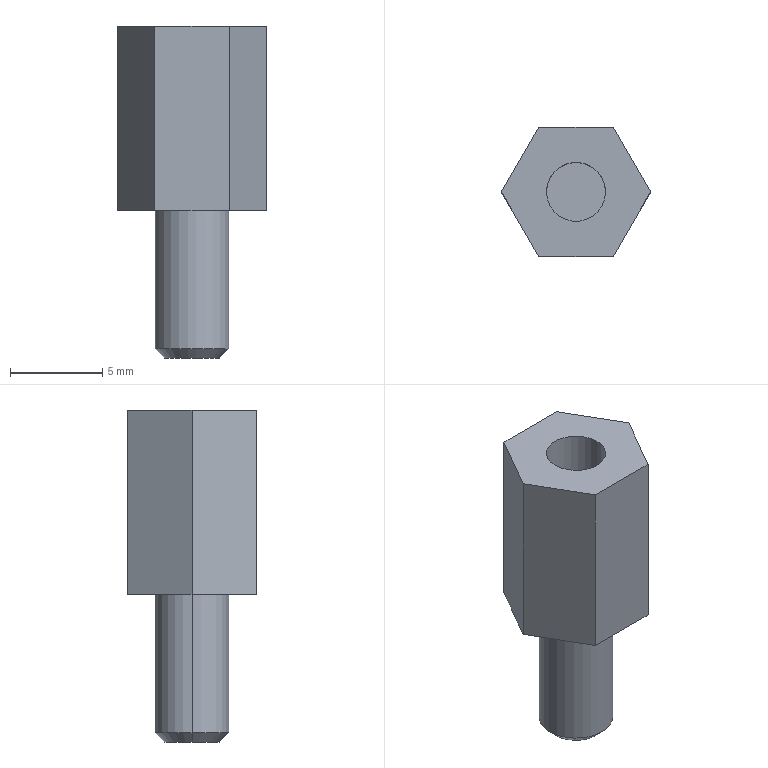Part | STEP file | 58411934 | 1 solid | 16 faces | box 8.091 x 7 x 18 mm | volume 467.745 mm3 | plane 10 | cylinder 4 | cone 2 | commonest cylinder face diameters 3.2 x2 4 x2
STEP:
#1=CARTESIAN_POINT('',(0.,0.,0.));
#2=DIRECTION('',(0.,0.,1.));
#3=DIRECTION('',(1.,0.,0.));
#4=AXIS2_PLACEMENT_3D('',#1,#2,#3);
#5=CARTESIAN_POINT('',(-2.025,3.5,0.));
#6=VERTEX_POINT('',#5);
#7=CARTESIAN_POINT('',(-4.046,0.,0.));
#8=VERTEX_POINT('',#7);
#9=CARTESIAN_POINT('',(-2.025,3.5,0.));
#10=DIRECTION('',(-0.5,-0.866,0.));
#11=VECTOR('',#10,1.);
#12=LINE('',#9,#11);
#13=CARTESIAN_POINT('',(0.,0.,0.));
#14=DIRECTION('',(0.,0.,1.));
#15=DIRECTION('',(1.,0.,0.));
#16=AXIS2_PLACEMENT_3D('',#13,#14,#15);
#17=PLANE('',#16);
#18=CARTESIAN_POINT('',(-2.025,3.5));
#19=DIRECTION('',(-0.5,-0.866));
#20=VECTOR('',#19,1.);
#21=LINE('',#18,#20);
#22=(GEOMETRIC_REPRESENTATION_CONTEXT(2)PARAMETRIC_REPRESENTATION_CONTEXT()REPRESENTATION_CONTEXT('',''));
#23=DEFINITIONAL_REPRESENTATION('',(#21),#22);
#24=PCURVE('',#17,#23);
#25=CARTESIAN_POINT('',(-2.025,3.5,0.));
#26=DIRECTION('',(-0.866,0.5,0.));
#27=DIRECTION('',(-0.5,-0.866,0.));
#28=AXIS2_PLACEMENT_3D('',#25,#26,#27);
#29=PLANE('',#28);
#30=CARTESIAN_POINT('',(0.,0.));
#31=DIRECTION('',(1.,0.));
#32=VECTOR('',#31,1.);
#33=LINE('',#30,#32);
#34=(GEOMETRIC_REPRESENTATION_CONTEXT(2)PARAMETRIC_REPRESENTATION_CONTEXT()REPRESENTATION_CONTEXT('',''));
#35=DEFINITIONAL_REPRESENTATION('',(#33),#34);
#36=PCURVE('',#29,#35);
#37=SURFACE_CURVE('',#12,(#24,#36),.PCURVE_S1.);
#38=EDGE_CURVE('',#6,#8,#37,.T.);
#39=ORIENTED_EDGE('',*,*,#38,.T.);
#40=CARTESIAN_POINT('',(-2.025,-3.5,0.));
#41=VERTEX_POINT('',#40);
#42=CARTESIAN_POINT('',(-2.025,-3.5,0.));
#43=DIRECTION('',(-0.5,0.866,0.));
#44=VECTOR('',#43,1.);
#45=LINE('',#42,#44);
#46=CARTESIAN_POINT('',(-2.025,-3.5));
#47=DIRECTION('',(-0.5,0.866));
#48=VECTOR('',#47,1.);
#49=LINE('',#46,#48);
#50=(GEOMETRIC_REPRESENTATION_CONTEXT(2)PARAMETRIC_REPRESENTATION_CONTEXT()REPRESENTATION_CONTEXT('',''));
#51=DEFINITIONAL_REPRESENTATION('',(#49),#50);
#52=PCURVE('',#17,#51);
#53=CARTESIAN_POINT('',(-2.025,-3.5,0.));
#54=DIRECTION('',(0.866,0.5,0.));
#55=DIRECTION('',(-0.5,0.866,0.));
#56=AXIS2_PLACEMENT_3D('',#53,#54,#55);
#57=PLANE('',#56);
#58=CARTESIAN_POINT('',(0.,0.));
#59=DIRECTION('',(1.,0.));
#60=VECTOR('',#59,1.);
#61=LINE('',#58,#60);
#62=(GEOMETRIC_REPRESENTATION_CONTEXT(2)PARAMETRIC_REPRESENTATION_CONTEXT()REPRESENTATION_CONTEXT('',''));
#63=DEFINITIONAL_REPRESENTATION('',(#61),#62);
#64=PCURVE('',#57,#63);
#65=SURFACE_CURVE('',#45,(#52,#64),.PCURVE_S1.);
#66=EDGE_CURVE('',#41,#8,#65,.T.);
#67=ORIENTED_EDGE('',*,*,#66,.F.);
#68=CARTESIAN_POINT('',(2.025,-3.5,0.));
#69=VERTEX_POINT('',#68);
#70=CARTESIAN_POINT('',(2.025,-3.5,0.));
#71=DIRECTION('',(-1.,0.,0.));
#72=VECTOR('',#71,1.);
#73=LINE('',#70,#72);
#74=CARTESIAN_POINT('',(2.025,-3.5));
#75=DIRECTION('',(-1.,0.));
#76=VECTOR('',#75,1.);
#77=LINE('',#74,#76);
#78=(GEOMETRIC_REPRESENTATION_CONTEXT(2)PARAMETRIC_REPRESENTATION_CONTEXT()REPRESENTATION_CONTEXT('',''));
#79=DEFINITIONAL_REPRESENTATION('',(#77),#78);
#80=PCURVE('',#17,#79);
#81=CARTESIAN_POINT('',(2.025,-3.5,0.));
#82=DIRECTION('',(0.,1.,0.));
#83=DIRECTION('',(-1.,0.,0.));
#84=AXIS2_PLACEMENT_3D('',#81,#82,#83);
#85=PLANE('',#84);
#86=CARTESIAN_POINT('',(0.,0.));
#87=DIRECTION('',(1.,0.));
#88=VECTOR('',#87,1.);
#89=LINE('',#86,#88);
#90=(GEOMETRIC_REPRESENTATION_CONTEXT(2)PARAMETRIC_REPRESENTATION_CONTEXT()REPRESENTATION_CONTEXT('',''));
#91=DEFINITIONAL_REPRESENTATION('',(#89),#90);
#92=PCURVE('',#85,#91);
#93=SURFACE_CURVE('',#73,(#80,#92),.PCURVE_S1.);
#94=EDGE_CURVE('',#69,#41,#93,.T.);
#95=ORIENTED_EDGE('',*,*,#94,.F.);
#96=CARTESIAN_POINT('',(4.046,0.,0.));
#97=VERTEX_POINT('',#96);
#98=CARTESIAN_POINT('',(4.046,0.,0.));
#99=DIRECTION('',(-0.5,-0.866,0.));
#100=VECTOR('',#99,1.);
#101=LINE('',#98,#100);
#102=CARTESIAN_POINT('',(4.046,0.));
#103=DIRECTION('',(-0.5,-0.866));
#104=VECTOR('',#103,1.);
#105=LINE('',#102,#104);
#106=(GEOMETRIC_REPRESENTATION_CONTEXT(2)PARAMETRIC_REPRESENTATION_CONTEXT()REPRESENTATION_CONTEXT('',''));
#107=DEFINITIONAL_REPRESENTATION('',(#105),#106);
#108=PCURVE('',#17,#107);
#109=CARTESIAN_POINT('',(4.046,0.,0.));
#110=DIRECTION('',(-0.866,0.5,0.));
#111=DIRECTION('',(-0.5,-0.866,0.));
#112=AXIS2_PLACEMENT_3D('',#109,#110,#111);
#113=PLANE('',#112);
#114=CARTESIAN_POINT('',(0.,0.));
#115=DIRECTION('',(1.,0.));
#116=VECTOR('',#115,1.);
#117=LINE('',#114,#116);
#118=(GEOMETRIC_REPRESENTATION_CONTEXT(2)PARAMETRIC_REPRESENTATION_CONTEXT()REPRESENTATION_CONTEXT('',''));
#119=DEFINITIONAL_REPRESENTATION('',(#117),#118);
#120=PCURVE('',#113,#119);
#121=SURFACE_CURVE('',#101,(#108,#120),.PCURVE_S1.);
#122=EDGE_CURVE('',#97,#69,#121,.T.);
#123=ORIENTED_EDGE('',*,*,#122,.F.);
#124=CARTESIAN_POINT('',(2.025,3.5,0.));
#125=VERTEX_POINT('',#124);
#126=CARTESIAN_POINT('',(4.046,0.,0.));
#127=DIRECTION('',(-0.5,0.866,0.));
#128=VECTOR('',#127,1.);
#129=LINE('',#126,#128);
#130=CARTESIAN_POINT('',(4.046,0.));
#131=DIRECTION('',(-0.5,0.866));
#132=VECTOR('',#131,1.);
#133=LINE('',#130,#132);
#134=(GEOMETRIC_REPRESENTATION_CONTEXT(2)PARAMETRIC_REPRESENTATION_CONTEXT()REPRESENTATION_CONTEXT('',''));
#135=DEFINITIONAL_REPRESENTATION('',(#133),#134);
#136=PCURVE('',#17,#135);
#137=CARTESIAN_POINT('',(4.046,0.,0.));
#138=DIRECTION('',(0.866,0.5,0.));
#139=DIRECTION('',(-0.5,0.866,0.));
#140=AXIS2_PLACEMENT_3D('',#137,#138,#139);
#141=PLANE('',#140);
#142=CARTESIAN_POINT('',(0.,0.));
#143=DIRECTION('',(1.,0.));
#144=VECTOR('',#143,1.);
#145=LINE('',#142,#144);
#146=(GEOMETRIC_REPRESENTATION_CONTEXT(2)PARAMETRIC_REPRESENTATION_CONTEXT()REPRESENTATION_CONTEXT('',''));
#147=DEFINITIONAL_REPRESENTATION('',(#145),#146);
#148=PCURVE('',#141,#147);
#149=SURFACE_CURVE('',#129,(#136,#148),.PCURVE_S1.);
#150=EDGE_CURVE('',#97,#125,#149,.T.);
#151=ORIENTED_EDGE('',*,*,#150,.T.);
#152=CARTESIAN_POINT('',(2.025,3.5,0.));
#153=DIRECTION('',(-1.,0.,0.));
#154=VECTOR('',#153,1.);
#155=LINE('',#152,#154);
#156=CARTESIAN_POINT('',(2.025,3.5));
#157=DIRECTION('',(-1.,0.));
#158=VECTOR('',#157,1.);
#159=LINE('',#156,#158);
#160=(GEOMETRIC_REPRESENTATION_CONTEXT(2)PARAMETRIC_REPRESENTATION_CONTEXT()REPRESENTATION_CONTEXT('',''));
#161=DEFINITIONAL_REPRESENTATION('',(#159),#160);
#162=PCURVE('',#17,#161);
#163=CARTESIAN_POINT('',(2.025,3.5,0.));
#164=DIRECTION('',(0.,1.,0.));
#165=DIRECTION('',(-1.,0.,0.));
#166=AXIS2_PLACEMENT_3D('',#163,#164,#165);
#167=PLANE('',#166);
#168=CARTESIAN_POINT('',(0.,0.));
#169=DIRECTION('',(1.,0.));
#170=VECTOR('',#169,1.);
#171=LINE('',#168,#170);
#172=(GEOMETRIC_REPRESENTATION_CONTEXT(2)PARAMETRIC_REPRESENTATION_CONTEXT()REPRESENTATION_CONTEXT('',''));
#173=DEFINITIONAL_REPRESENTATION('',(#171),#172);
#174=PCURVE('',#167,#173);
#175=SURFACE_CURVE('',#155,(#162,#174),.PCURVE_S1.);
#176=EDGE_CURVE('',#125,#6,#175,.T.);
#177=ORIENTED_EDGE('',*,*,#176,.T.);
#178=EDGE_LOOP('',(#39,#67,#95,#123,#151,#177));
#179=FACE_BOUND('',#178,.F.);
#180=CARTESIAN_POINT('',(-2.,0.,0.));
#181=VERTEX_POINT('',#180);
#182=CARTESIAN_POINT('',(2.,0.,0.));
#183=VERTEX_POINT('',#182);
#184=CARTESIAN_POINT('',(0.,0.,0.));
#185=DIRECTION('',(0.,0.,-1.));
#186=DIRECTION('',(-1.,0.,0.));
#187=AXIS2_PLACEMENT_3D('',#184,#185,#186);
#188=CIRCLE('',#187,2.);
#189=CARTESIAN_POINT('',(-2.,0.));
#190=CARTESIAN_POINT('',(-2.,3.464));
#191=CARTESIAN_POINT('',(1.,1.732));
#192=CARTESIAN_POINT('',(4.,0.));
#193=CARTESIAN_POINT('',(1.,-1.732));
#194=CARTESIAN_POINT('',(-2.,-3.464));
#195=CARTESIAN_POINT('',(-2.,0.));
#196=(BOUNDED_CURVE()B_SPLINE_CURVE(2,(#189,#190,#191,#192,#193,#194,#195),.UNSPECIFIED.,.T.,.F.)B_SPLINE_CURVE_WITH_KNOTS((1,2,2,2,2,1),(-2.094,0.,2.094,4.189,6.283,8.378),.UNSPECIFIED.)CURVE()GEOMETRIC_REPRESENTATION_ITEM()RATIONAL_B_SPLINE_CURVE((1.,0.5,1.,0.5,1.,0.5,1.))REPRESENTATION_ITEM(''));
#197=(GEOMETRIC_REPRESENTATION_CONTEXT(2)PARAMETRIC_REPRESENTATION_CONTEXT()REPRESENTATION_CONTEXT('',''));
#198=DEFINITIONAL_REPRESENTATION('',(#196),#197);
#199=PCURVE('',#17,#198);
#200=CARTESIAN_POINT('',(0.,0.,0.));
#201=DIRECTION('',(0.,0.,-1.));
#202=DIRECTION('',(-1.,0.,0.));
#203=AXIS2_PLACEMENT_3D('',#200,#201,#202);
#204=CYLINDRICAL_SURFACE('',#203,2.);
#205=CARTESIAN_POINT('',(0.,0.));
#206=DIRECTION('',(1.,0.));
#207=VECTOR('',#206,1.);
#208=LINE('',#205,#207);
#209=(GEOMETRIC_REPRESENTATION_CONTEXT(2)PARAMETRIC_REPRESENTATION_CONTEXT()REPRESENTATION_CONTEXT('',''));
#210=DEFINITIONAL_REPRESENTATION('',(#208),#209);
#211=PCURVE('',#204,#210);
#212=SURFACE_CURVE('',#188,(#199,#211),.PCURVE_S1.);
#213=EDGE_CURVE('',#181,#183,#212,.T.);
#214=ORIENTED_EDGE('',*,*,#213,.T.);
#215=CARTESIAN_POINT('',(0.,0.,0.));
#216=DIRECTION('',(0.,0.,-1.));
#217=DIRECTION('',(1.,0.,0.));
#218=AXIS2_PLACEMENT_3D('',#215,#216,#217);
#219=CIRCLE('',#218,2.);
#220=CARTESIAN_POINT('',(2.,0.));
#221=CARTESIAN_POINT('',(2.,-3.464));
#222=CARTESIAN_POINT('',(-1.,-1.732));
#223=CARTESIAN_POINT('',(-4.,0.));
#224=CARTESIAN_POINT('',(-1.,1.732));
#225=CARTESIAN_POINT('',(2.,3.464));
#226=CARTESIAN_POINT('',(2.,0.));
#227=(BOUNDED_CURVE()B_SPLINE_CURVE(2,(#220,#221,#222,#223,#224,#225,#226),.UNSPECIFIED.,.T.,.F.)B_SPLINE_CURVE_WITH_KNOTS((1,2,2,2,2,1),(-2.094,0.,2.094,4.189,6.283,8.378),.UNSPECIFIED.)CURVE()GEOMETRIC_REPRESENTATION_ITEM()RATIONAL_B_SPLINE_CURVE((1.,0.5,1.,0.5,1.,0.5,1.))REPRESENTATION_ITEM(''));
#228=(GEOMETRIC_REPRESENTATION_CONTEXT(2)PARAMETRIC_REPRESENTATION_CONTEXT()REPRESENTATION_CONTEXT('',''));
#229=DEFINITIONAL_REPRESENTATION('',(#227),#228);
#230=PCURVE('',#17,#229);
#231=CARTESIAN_POINT('',(0.,0.,0.));
#232=DIRECTION('',(0.,0.,-1.));
#233=DIRECTION('',(-1.,0.,0.));
#234=AXIS2_PLACEMENT_3D('',#231,#232,#233);
#235=CYLINDRICAL_SURFACE('',#234,2.);
#236=CARTESIAN_POINT('',(3.142,0.));
#237=DIRECTION('',(1.,0.));
#238=VECTOR('',#237,1.);
#239=LINE('',#236,#238);
#240=(GEOMETRIC_REPRESENTATION_CONTEXT(2)PARAMETRIC_REPRESENTATION_CONTEXT()REPRESENTATION_CONTEXT('',''));
#241=DEFINITIONAL_REPRESENTATION('',(#239),#240);
#242=PCURVE('',#235,#241);
#243=SURFACE_CURVE('',#219,(#230,#242),.PCURVE_S1.);
#244=EDGE_CURVE('',#183,#181,#243,.T.);
#245=ORIENTED_EDGE('',*,*,#244,.T.);
#246=EDGE_LOOP('',(#214,#245));
#247=FACE_BOUND('',#246,.F.);
#248=ADVANCED_FACE('',(#179,#247),#17,.F.);
#249=CARTESIAN_POINT('',(-4.046,0.,10.));
#250=VERTEX_POINT('',#249);
#251=CARTESIAN_POINT('',(-4.046,0.,0.));
#252=DIRECTION('',(0.,0.,1.));
#253=VECTOR('',#252,1.);
#254=LINE('',#251,#253);
#255=CARTESIAN_POINT('',(4.041,0.));
#256=DIRECTION('',(0.,1.));
#257=VECTOR('',#256,1.);
#258=LINE('',#255,#257);
#259=(GEOMETRIC_REPRESENTATION_CONTEXT(2)PARAMETRIC_REPRESENTATION_CONTEXT()REPRESENTATION_CONTEXT('',''));
#260=DEFINITIONAL_REPRESENTATION('',(#258),#259);
#261=PCURVE('',#29,#260);
#262=CARTESIAN_POINT('',(4.041,0.));
#263=DIRECTION('',(0.,1.));
#264=VECTOR('',#263,1.);
#265=LINE('',#262,#264);
#266=(GEOMETRIC_REPRESENTATION_CONTEXT(2)PARAMETRIC_REPRESENTATION_CONTEXT()REPRESENTATION_CONTEXT('',''));
#267=DEFINITIONAL_REPRESENTATION('',(#265),#266);
#268=PCURVE('',#57,#267);
#269=SURFACE_CURVE('',#254,(#261,#268),.PCURVE_S1.);
#270=EDGE_CURVE('',#8,#250,#269,.T.);
#271=ORIENTED_EDGE('',*,*,#270,.F.);
#272=ORIENTED_EDGE('',*,*,#38,.F.);
#273=CARTESIAN_POINT('',(-2.025,3.5,10.));
#274=VERTEX_POINT('',#273);
#275=CARTESIAN_POINT('',(-2.025,3.5,0.));
#276=DIRECTION('',(0.,0.,1.));
#277=VECTOR('',#276,1.);
#278=LINE('',#275,#277);
#279=CARTESIAN_POINT('',(0.,0.));
#280=DIRECTION('',(0.,1.));
#281=VECTOR('',#280,1.);
#282=LINE('',#279,#281);
#283=(GEOMETRIC_REPRESENTATION_CONTEXT(2)PARAMETRIC_REPRESENTATION_CONTEXT()REPRESENTATION_CONTEXT('',''));
#284=DEFINITIONAL_REPRESENTATION('',(#282),#283);
#285=PCURVE('',#29,#284);
#286=CARTESIAN_POINT('',(4.05,0.));
#287=DIRECTION('',(0.,1.));
#288=VECTOR('',#287,1.);
#289=LINE('',#286,#288);
#290=(GEOMETRIC_REPRESENTATION_CONTEXT(2)PARAMETRIC_REPRESENTATION_CONTEXT()REPRESENTATION_CONTEXT('',''));
#291=DEFINITIONAL_REPRESENTATION('',(#289),#290);
#292=PCURVE('',#167,#291);
#293=SURFACE_CURVE('',#278,(#285,#292),.PCURVE_S1.);
#294=EDGE_CURVE('',#6,#274,#293,.T.);
#295=ORIENTED_EDGE('',*,*,#294,.T.);
#296=CARTESIAN_POINT('',(-2.025,3.5,10.));
#297=DIRECTION('',(-0.5,-0.866,0.));
#298=VECTOR('',#297,1.);
#299=LINE('',#296,#298);
#300=CARTESIAN_POINT('',(0.,10.));
#301=DIRECTION('',(1.,0.));
#302=VECTOR('',#301,1.);
#303=LINE('',#300,#302);
#304=(GEOMETRIC_REPRESENTATION_CONTEXT(2)PARAMETRIC_REPRESENTATION_CONTEXT()REPRESENTATION_CONTEXT('',''));
#305=DEFINITIONAL_REPRESENTATION('',(#303),#304);
#306=PCURVE('',#29,#305);
#307=CARTESIAN_POINT('',(0.,0.,10.));
#308=DIRECTION('',(0.,0.,1.));
#309=DIRECTION('',(1.,0.,0.));
#310=AXIS2_PLACEMENT_3D('',#307,#308,#309);
#311=PLANE('',#310);
#312=CARTESIAN_POINT('',(-2.025,3.5));
#313=DIRECTION('',(-0.5,-0.866));
#314=VECTOR('',#313,1.);
#315=LINE('',#312,#314);
#316=(GEOMETRIC_REPRESENTATION_CONTEXT(2)PARAMETRIC_REPRESENTATION_CONTEXT()REPRESENTATION_CONTEXT('',''));
#317=DEFINITIONAL_REPRESENTATION('',(#315),#316);
#318=PCURVE('',#311,#317);
#319=SURFACE_CURVE('',#299,(#306,#318),.PCURVE_S1.);
#320=EDGE_CURVE('',#274,#250,#319,.T.);
#321=ORIENTED_EDGE('',*,*,#320,.T.);
#322=EDGE_LOOP('',(#271,#272,#295,#321));
#323=FACE_BOUND('',#322,.F.);
#324=ADVANCED_FACE('',(#323),#29,.T.);
#325=ORIENTED_EDGE('',*,*,#270,.T.);
#326=CARTESIAN_POINT('',(-2.025,-3.5,10.));
#327=VERTEX_POINT('',#326);
#328=CARTESIAN_POINT('',(-2.025,-3.5,10.));
#329=DIRECTION('',(-0.5,0.866,0.));
#330=VECTOR('',#329,1.);
#331=LINE('',#328,#330);
#332=CARTESIAN_POINT('',(0.,10.));
#333=DIRECTION('',(1.,0.));
#334=VECTOR('',#333,1.);
#335=LINE('',#332,#334);
#336=(GEOMETRIC_REPRESENTATION_CONTEXT(2)PARAMETRIC_REPRESENTATION_CONTEXT()REPRESENTATION_CONTEXT('',''));
#337=DEFINITIONAL_REPRESENTATION('',(#335),#336);
#338=PCURVE('',#57,#337);
#339=CARTESIAN_POINT('',(-2.025,-3.5));
#340=DIRECTION('',(-0.5,0.866));
#341=VECTOR('',#340,1.);
#342=LINE('',#339,#341);
#343=(GEOMETRIC_REPRESENTATION_CONTEXT(2)PARAMETRIC_REPRESENTATION_CONTEXT()REPRESENTATION_CONTEXT('',''));
#344=DEFINITIONAL_REPRESENTATION('',(#342),#343);
#345=PCURVE('',#311,#344);
#346=SURFACE_CURVE('',#331,(#338,#345),.PCURVE_S1.);
#347=EDGE_CURVE('',#327,#250,#346,.T.);
#348=ORIENTED_EDGE('',*,*,#347,.F.);
#349=CARTESIAN_POINT('',(-2.025,-3.5,0.));
#350=DIRECTION('',(0.,0.,1.));
#351=VECTOR('',#350,1.);
#352=LINE('',#349,#351);
#353=CARTESIAN_POINT('',(0.,0.));
#354=DIRECTION('',(0.,1.));
#355=VECTOR('',#354,1.);
#356=LINE('',#353,#355);
#357=(GEOMETRIC_REPRESENTATION_CONTEXT(2)PARAMETRIC_REPRESENTATION_CONTEXT()REPRESENTATION_CONTEXT('',''));
#358=DEFINITIONAL_REPRESENTATION('',(#356),#357);
#359=PCURVE('',#57,#358);
#360=CARTESIAN_POINT('',(4.05,0.));
#361=DIRECTION('',(0.,1.));
#362=VECTOR('',#361,1.);
#363=LINE('',#360,#362);
#364=(GEOMETRIC_REPRESENTATION_CONTEXT(2)PARAMETRIC_REPRESENTATION_CONTEXT()REPRESENTATION_CONTEXT('',''));
#365=DEFINITIONAL_REPRESENTATION('',(#363),#364);
#366=PCURVE('',#85,#365);
#367=SURFACE_CURVE('',#352,(#359,#366),.PCURVE_S1.);
#368=EDGE_CURVE('',#41,#327,#367,.T.);
#369=ORIENTED_EDGE('',*,*,#368,.F.);
#370=ORIENTED_EDGE('',*,*,#66,.T.);
#371=EDGE_LOOP('',(#325,#348,#369,#370));
#372=FACE_BOUND('',#371,.F.);
#373=ADVANCED_FACE('',(#372),#57,.F.);
#374=CARTESIAN_POINT('',(4.046,0.,10.));
#375=VERTEX_POINT('',#374);
#376=CARTESIAN_POINT('',(2.025,3.5,10.));
#377=VERTEX_POINT('',#376);
#378=CARTESIAN_POINT('',(4.046,0.,10.));
#379=DIRECTION('',(-0.5,0.866,0.));
#380=VECTOR('',#379,1.);
#381=LINE('',#378,#380);
#382=CARTESIAN_POINT('',(4.046,0.));
#383=DIRECTION('',(-0.5,0.866));
#384=VECTOR('',#383,1.);
#385=LINE('',#382,#384);
#386=(GEOMETRIC_REPRESENTATION_CONTEXT(2)PARAMETRIC_REPRESENTATION_CONTEXT()REPRESENTATION_CONTEXT('',''));
#387=DEFINITIONAL_REPRESENTATION('',(#385),#386);
#388=PCURVE('',#311,#387);
#389=CARTESIAN_POINT('',(0.,10.));
#390=DIRECTION('',(1.,0.));
#391=VECTOR('',#390,1.);
#392=LINE('',#389,#391);
#393=(GEOMETRIC_REPRESENTATION_CONTEXT(2)PARAMETRIC_REPRESENTATION_CONTEXT()REPRESENTATION_CONTEXT('',''));
#394=DEFINITIONAL_REPRESENTATION('',(#392),#393);
#395=PCURVE('',#141,#394);
#396=SURFACE_CURVE('',#381,(#388,#395),.PCURVE_S1.);
#397=EDGE_CURVE('',#375,#377,#396,.T.);
#398=ORIENTED_EDGE('',*,*,#397,.F.);
#399=CARTESIAN_POINT('',(2.025,-3.5,10.));
#400=VERTEX_POINT('',#399);
#401=CARTESIAN_POINT('',(4.046,0.,10.));
#402=DIRECTION('',(-0.5,-0.866,0.));
#403=VECTOR('',#402,1.);
#404=LINE('',#401,#403);
#405=CARTESIAN_POINT('',(4.046,0.));
#406=DIRECTION('',(-0.5,-0.866));
#407=VECTOR('',#406,1.);
#408=LINE('',#405,#407);
#409=(GEOMETRIC_REPRESENTATION_CONTEXT(2)PARAMETRIC_REPRESENTATION_CONTEXT()REPRESENTATION_CONTEXT('',''));
#410=DEFINITIONAL_REPRESENTATION('',(#408),#409);
#411=PCURVE('',#311,#410);
#412=CARTESIAN_POINT('',(0.,10.));
#413=DIRECTION('',(1.,0.));
#414=VECTOR('',#413,1.);
#415=LINE('',#412,#414);
#416=(GEOMETRIC_REPRESENTATION_CONTEXT(2)PARAMETRIC_REPRESENTATION_CONTEXT()REPRESENTATION_CONTEXT('',''));
#417=DEFINITIONAL_REPRESENTATION('',(#415),#416);
#418=PCURVE('',#113,#417);
#419=SURFACE_CURVE('',#404,(#411,#418),.PCURVE_S1.);
#420=EDGE_CURVE('',#375,#400,#419,.T.);
#421=ORIENTED_EDGE('',*,*,#420,.T.);
#422=CARTESIAN_POINT('',(2.025,-3.5,10.));
#423=DIRECTION('',(-1.,0.,0.));
#424=VECTOR('',#423,1.);
#425=LINE('',#422,#424);
#426=CARTESIAN_POINT('',(2.025,-3.5));
#427=DIRECTION('',(-1.,0.));
#428=VECTOR('',#427,1.);
#429=LINE('',#426,#428);
#430=(GEOMETRIC_REPRESENTATION_CONTEXT(2)PARAMETRIC_REPRESENTATION_CONTEXT()REPRESENTATION_CONTEXT('',''));
#431=DEFINITIONAL_REPRESENTATION('',(#429),#430);
#432=PCURVE('',#311,#431);
#433=CARTESIAN_POINT('',(0.,10.));
#434=DIRECTION('',(1.,0.));
#435=VECTOR('',#434,1.);
#436=LINE('',#433,#435);
#437=(GEOMETRIC_REPRESENTATION_CONTEXT(2)PARAMETRIC_REPRESENTATION_CONTEXT()REPRESENTATION_CONTEXT('',''));
#438=DEFINITIONAL_REPRESENTATION('',(#436),#437);
#439=PCURVE('',#85,#438);
#440=SURFACE_CURVE('',#425,(#432,#439),.PCURVE_S1.);
#441=EDGE_CURVE('',#400,#327,#440,.T.);
#442=ORIENTED_EDGE('',*,*,#441,.T.);
#443=ORIENTED_EDGE('',*,*,#347,.T.);
#444=ORIENTED_EDGE('',*,*,#320,.F.);
#445=CARTESIAN_POINT('',(2.025,3.5,10.));
#446=DIRECTION('',(-1.,0.,0.));
#447=VECTOR('',#446,1.);
#448=LINE('',#445,#447);
#449=CARTESIAN_POINT('',(2.025,3.5));
#450=DIRECTION('',(-1.,0.));
#451=VECTOR('',#450,1.);
#452=LINE('',#449,#451);
#453=(GEOMETRIC_REPRESENTATION_CONTEXT(2)PARAMETRIC_REPRESENTATION_CONTEXT()REPRESENTATION_CONTEXT('',''));
#454=DEFINITIONAL_REPRESENTATION('',(#452),#453);
#455=PCURVE('',#311,#454);
#456=CARTESIAN_POINT('',(0.,10.));
#457=DIRECTION('',(1.,0.));
#458=VECTOR('',#457,1.);
#459=LINE('',#456,#458);
#460=(GEOMETRIC_REPRESENTATION_CONTEXT(2)PARAMETRIC_REPRESENTATION_CONTEXT()REPRESENTATION_CONTEXT('',''));
#461=DEFINITIONAL_REPRESENTATION('',(#459),#460);
#462=PCURVE('',#167,#461);
#463=SURFACE_CURVE('',#448,(#455,#462),.PCURVE_S1.);
#464=EDGE_CURVE('',#377,#274,#463,.T.);
#465=ORIENTED_EDGE('',*,*,#464,.F.);
#466=EDGE_LOOP('',(#398,#421,#442,#443,#444,#465));
#467=FACE_BOUND('',#466,.F.);
#468=CARTESIAN_POINT('',(-1.6,0.,10.));
#469=VERTEX_POINT('',#468);
#470=CARTESIAN_POINT('',(1.6,0.,10.));
#471=VERTEX_POINT('',#470);
#472=CARTESIAN_POINT('',(0.,0.,10.));
#473=DIRECTION('',(0.,0.,-1.));
#474=DIRECTION('',(-1.,0.,0.));
#475=AXIS2_PLACEMENT_3D('',#472,#473,#474);
#476=CIRCLE('',#475,1.6);
#477=CARTESIAN_POINT('',(-1.6,0.));
#478=CARTESIAN_POINT('',(-1.6,2.771));
#479=CARTESIAN_POINT('',(0.8,1.386));
#480=CARTESIAN_POINT('',(3.2,0.));
#481=CARTESIAN_POINT('',(0.8,-1.386));
#482=CARTESIAN_POINT('',(-1.6,-2.771));
#483=CARTESIAN_POINT('',(-1.6,0.));
#484=(BOUNDED_CURVE()B_SPLINE_CURVE(2,(#477,#478,#479,#480,#481,#482,#483),.UNSPECIFIED.,.T.,.F.)B_SPLINE_CURVE_WITH_KNOTS((1,2,2,2,2,1),(-2.094,0.,2.094,4.189,6.283,8.378),.UNSPECIFIED.)CURVE()GEOMETRIC_REPRESENTATION_ITEM()RATIONAL_B_SPLINE_CURVE((1.,0.5,1.,0.5,1.,0.5,1.))REPRESENTATION_ITEM(''));
#485=(GEOMETRIC_REPRESENTATION_CONTEXT(2)PARAMETRIC_REPRESENTATION_CONTEXT()REPRESENTATION_CONTEXT('',''));
#486=DEFINITIONAL_REPRESENTATION('',(#484),#485);
#487=PCURVE('',#311,#486);
#488=CARTESIAN_POINT('',(0.,0.,10.));
#489=DIRECTION('',(0.,0.,-1.));
#490=DIRECTION('',(-1.,0.,0.));
#491=AXIS2_PLACEMENT_3D('',#488,#489,#490);
#492=CYLINDRICAL_SURFACE('',#491,1.6);
#493=CARTESIAN_POINT('',(0.,0.));
#494=DIRECTION('',(1.,0.));
#495=VECTOR('',#494,1.);
#496=LINE('',#493,#495);
#497=(GEOMETRIC_REPRESENTATION_CONTEXT(2)PARAMETRIC_REPRESENTATION_CONTEXT()REPRESENTATION_CONTEXT('',''));
#498=DEFINITIONAL_REPRESENTATION('',(#496),#497);
#499=PCURVE('',#492,#498);
#500=SURFACE_CURVE('',#476,(#487,#499),.PCURVE_S1.);
#501=EDGE_CURVE('',#469,#471,#500,.T.);
#502=ORIENTED_EDGE('',*,*,#501,.F.);
#503=CARTESIAN_POINT('',(0.,0.,10.));
#504=DIRECTION('',(0.,0.,-1.));
#505=DIRECTION('',(1.,0.,0.));
#506=AXIS2_PLACEMENT_3D('',#503,#504,#505);
#507=CIRCLE('',#506,1.6);
#508=CARTESIAN_POINT('',(1.6,0.));
#509=CARTESIAN_POINT('',(1.6,-2.771));
#510=CARTESIAN_POINT('',(-0.8,-1.386));
#511=CARTESIAN_POINT('',(-3.2,0.));
#512=CARTESIAN_POINT('',(-0.8,1.386));
#513=CARTESIAN_POINT('',(1.6,2.771));
#514=CARTESIAN_POINT('',(1.6,0.));
#515=(BOUNDED_CURVE()B_SPLINE_CURVE(2,(#508,#509,#510,#511,#512,#513,#514),.UNSPECIFIED.,.T.,.F.)B_SPLINE_CURVE_WITH_KNOTS((1,2,2,2,2,1),(-2.094,0.,2.094,4.189,6.283,8.378),.UNSPECIFIED.)CURVE()GEOMETRIC_REPRESENTATION_ITEM()RATIONAL_B_SPLINE_CURVE((1.,0.5,1.,0.5,1.,0.5,1.))REPRESENTATION_ITEM(''));
#516=(GEOMETRIC_REPRESENTATION_CONTEXT(2)PARAMETRIC_REPRESENTATION_CONTEXT()REPRESENTATION_CONTEXT('',''));
#517=DEFINITIONAL_REPRESENTATION('',(#515),#516);
#518=PCURVE('',#311,#517);
#519=CARTESIAN_POINT('',(0.,0.,10.));
#520=DIRECTION('',(0.,0.,-1.));
#521=DIRECTION('',(-1.,0.,0.));
#522=AXIS2_PLACEMENT_3D('',#519,#520,#521);
#523=CYLINDRICAL_SURFACE('',#522,1.6);
#524=CARTESIAN_POINT('',(3.142,0.));
#525=DIRECTION('',(1.,0.));
#526=VECTOR('',#525,1.);
#527=LINE('',#524,#526);
#528=(GEOMETRIC_REPRESENTATION_CONTEXT(2)PARAMETRIC_REPRESENTATION_CONTEXT()REPRESENTATION_CONTEXT('',''));
#529=DEFINITIONAL_REPRESENTATION('',(#527),#528);
#530=PCURVE('',#523,#529);
#531=SURFACE_CURVE('',#507,(#518,#530),.PCURVE_S1.);
#532=EDGE_CURVE('',#471,#469,#531,.T.);
#533=ORIENTED_EDGE('',*,*,#532,.F.);
#534=EDGE_LOOP('',(#502,#533));
#535=FACE_BOUND('',#534,.F.);
#536=ADVANCED_FACE('',(#467,#535),#311,.T.);
#537=CARTESIAN_POINT('',(4.046,0.,0.));
#538=DIRECTION('',(0.,0.,1.));
#539=VECTOR('',#538,1.);
#540=LINE('',#537,#539);
#541=CARTESIAN_POINT('',(0.,0.));
#542=DIRECTION('',(0.,1.));
#543=VECTOR('',#542,1.);
#544=LINE('',#541,#543);
#545=(GEOMETRIC_REPRESENTATION_CONTEXT(2)PARAMETRIC_REPRESENTATION_CONTEXT()REPRESENTATION_CONTEXT('',''));
#546=DEFINITIONAL_REPRESENTATION('',(#544),#545);
#547=PCURVE('',#141,#546);
#548=CARTESIAN_POINT('',(0.,0.));
#549=DIRECTION('',(0.,1.));
#550=VECTOR('',#549,1.);
#551=LINE('',#548,#550);
#552=(GEOMETRIC_REPRESENTATION_CONTEXT(2)PARAMETRIC_REPRESENTATION_CONTEXT()REPRESENTATION_CONTEXT('',''));
#553=DEFINITIONAL_REPRESENTATION('',(#551),#552);
#554=PCURVE('',#113,#553);
#555=SURFACE_CURVE('',#540,(#547,#554),.PCURVE_S1.);
#556=EDGE_CURVE('',#97,#375,#555,.T.);
#557=ORIENTED_EDGE('',*,*,#556,.T.);
#558=ORIENTED_EDGE('',*,*,#397,.T.);
#559=CARTESIAN_POINT('',(2.025,3.5,0.));
#560=DIRECTION('',(0.,0.,1.));
#561=VECTOR('',#560,1.);
#562=LINE('',#559,#561);
#563=CARTESIAN_POINT('',(4.041,0.));
#564=DIRECTION('',(0.,1.));
#565=VECTOR('',#564,1.);
#566=LINE('',#563,#565);
#567=(GEOMETRIC_REPRESENTATION_CONTEXT(2)PARAMETRIC_REPRESENTATION_CONTEXT()REPRESENTATION_CONTEXT('',''));
#568=DEFINITIONAL_REPRESENTATION('',(#566),#567);
#569=PCURVE('',#141,#568);
#570=CARTESIAN_POINT('',(0.,0.));
#571=DIRECTION('',(0.,1.));
#572=VECTOR('',#571,1.);
#573=LINE('',#570,#572);
#574=(GEOMETRIC_REPRESENTATION_CONTEXT(2)PARAMETRIC_REPRESENTATION_CONTEXT()REPRESENTATION_CONTEXT('',''));
#575=DEFINITIONAL_REPRESENTATION('',(#573),#574);
#576=PCURVE('',#167,#575);
#577=SURFACE_CURVE('',#562,(#569,#576),.PCURVE_S1.);
#578=EDGE_CURVE('',#125,#377,#577,.T.);
#579=ORIENTED_EDGE('',*,*,#578,.F.);
#580=ORIENTED_EDGE('',*,*,#150,.F.);
#581=EDGE_LOOP('',(#557,#558,#579,#580));
#582=FACE_BOUND('',#581,.F.);
#583=ADVANCED_FACE('',(#582),#141,.T.);
#584=ORIENTED_EDGE('',*,*,#556,.F.);
#585=ORIENTED_EDGE('',*,*,#122,.T.);
#586=CARTESIAN_POINT('',(2.025,-3.5,0.));
#587=DIRECTION('',(0.,0.,1.));
#588=VECTOR('',#587,1.);
#589=LINE('',#586,#588);
#590=CARTESIAN_POINT('',(4.041,0.));
#591=DIRECTION('',(0.,1.));
#592=VECTOR('',#591,1.);
#593=LINE('',#590,#592);
#594=(GEOMETRIC_REPRESENTATION_CONTEXT(2)PARAMETRIC_REPRESENTATION_CONTEXT()REPRESENTATION_CONTEXT('',''));
#595=DEFINITIONAL_REPRESENTATION('',(#593),#594);
#596=PCURVE('',#113,#595);
#597=CARTESIAN_POINT('',(0.,0.));
#598=DIRECTION('',(0.,1.));
#599=VECTOR('',#598,1.);
#600=LINE('',#597,#599);
#601=(GEOMETRIC_REPRESENTATION_CONTEXT(2)PARAMETRIC_REPRESENTATION_CONTEXT()REPRESENTATION_CONTEXT('',''));
#602=DEFINITIONAL_REPRESENTATION('',(#600),#601);
#603=PCURVE('',#85,#602);
#604=SURFACE_CURVE('',#589,(#596,#603),.PCURVE_S1.);
#605=EDGE_CURVE('',#69,#400,#604,.T.);
#606=ORIENTED_EDGE('',*,*,#605,.T.);
#607=ORIENTED_EDGE('',*,*,#420,.F.);
#608=EDGE_LOOP('',(#584,#585,#606,#607));
#609=FACE_BOUND('',#608,.F.);
#610=ADVANCED_FACE('',(#609),#113,.F.);
#611=ORIENTED_EDGE('',*,*,#94,.T.);
#612=ORIENTED_EDGE('',*,*,#368,.T.);
#613=ORIENTED_EDGE('',*,*,#441,.F.);
#614=ORIENTED_EDGE('',*,*,#605,.F.);
#615=EDGE_LOOP('',(#611,#612,#613,#614));
#616=FACE_BOUND('',#615,.F.);
#617=ADVANCED_FACE('',(#616),#85,.F.);
#618=ORIENTED_EDGE('',*,*,#176,.F.);
#619=ORIENTED_EDGE('',*,*,#578,.T.);
#620=ORIENTED_EDGE('',*,*,#464,.T.);
#621=ORIENTED_EDGE('',*,*,#294,.F.);
#622=EDGE_LOOP('',(#618,#619,#620,#621));
#623=FACE_BOUND('',#622,.F.);
#624=ADVANCED_FACE('',(#623),#167,.T.);
#625=ORIENTED_EDGE('',*,*,#501,.T.);
#626=CARTESIAN_POINT('',(1.6,0.,3.));
#627=VERTEX_POINT('',#626);
#628=CARTESIAN_POINT('',(1.6,0.,10.));
#629=DIRECTION('',(0.,0.,-1.));
#630=VECTOR('',#629,1.);
#631=LINE('',#628,#630);
#632=CARTESIAN_POINT('',(3.142,0.));
#633=DIRECTION('',(0.,1.));
#634=VECTOR('',#633,1.);
#635=LINE('',#632,#634);
#636=(GEOMETRIC_REPRESENTATION_CONTEXT(2)PARAMETRIC_REPRESENTATION_CONTEXT()REPRESENTATION_CONTEXT('',''));
#637=DEFINITIONAL_REPRESENTATION('',(#635),#636);
#638=PCURVE('',#492,#637);
#639=CARTESIAN_POINT('',(3.142,0.));
#640=DIRECTION('',(0.,1.));
#641=VECTOR('',#640,1.);
#642=LINE('',#639,#641);
#643=(GEOMETRIC_REPRESENTATION_CONTEXT(2)PARAMETRIC_REPRESENTATION_CONTEXT()REPRESENTATION_CONTEXT('',''));
#644=DEFINITIONAL_REPRESENTATION('',(#642),#643);
#645=PCURVE('',#523,#644);
#646=SURFACE_CURVE('',#631,(#638,#645),.PCURVE_S1.);
#647=EDGE_CURVE('',#471,#627,#646,.T.);
#648=ORIENTED_EDGE('',*,*,#647,.T.);
#649=CARTESIAN_POINT('',(-1.6,0.,3.));
#650=VERTEX_POINT('',#649);
#651=CARTESIAN_POINT('',(0.,0.,3.));
#652=DIRECTION('',(0.,0.,-1.));
#653=DIRECTION('',(-1.,0.,0.));
#654=AXIS2_PLACEMENT_3D('',#651,#652,#653);
#655=CIRCLE('',#654,1.6);
#656=CARTESIAN_POINT('',(0.,7.));
#657=DIRECTION('',(1.,0.));
#658=VECTOR('',#657,1.);
#659=LINE('',#656,#658);
#660=(GEOMETRIC_REPRESENTATION_CONTEXT(2)PARAMETRIC_REPRESENTATION_CONTEXT()REPRESENTATION_CONTEXT('',''));
#661=DEFINITIONAL_REPRESENTATION('',(#659),#660);
#662=PCURVE('',#492,#661);
#663=CARTESIAN_POINT('',(0.,0.,3.));
#664=DIRECTION('',(0.,0.,-1.));
#665=DIRECTION('',(-1.,0.,0.));
#666=AXIS2_PLACEMENT_3D('',#663,#664,#665);
#667=PLANE('',#666);
#668=CARTESIAN_POINT('',(0.,0.));
#669=DIRECTION('',(1.,0.));
#670=AXIS2_PLACEMENT_2D('',#668,#669);
#671=CIRCLE('',#670,1.6);
#672=(GEOMETRIC_REPRESENTATION_CONTEXT(2)PARAMETRIC_REPRESENTATION_CONTEXT()REPRESENTATION_CONTEXT('',''));
#673=DEFINITIONAL_REPRESENTATION('',(#671),#672);
#674=PCURVE('',#667,#673);
#675=SURFACE_CURVE('',#655,(#662,#674),.PCURVE_S1.);
#676=EDGE_CURVE('',#650,#627,#675,.T.);
#677=ORIENTED_EDGE('',*,*,#676,.F.);
#678=CARTESIAN_POINT('',(-1.6,0.,10.));
#679=DIRECTION('',(0.,0.,-1.));
#680=VECTOR('',#679,1.);
#681=LINE('',#678,#680);
#682=CARTESIAN_POINT('',(0.,0.));
#683=DIRECTION('',(0.,1.));
#684=VECTOR('',#683,1.);
#685=LINE('',#682,#684);
#686=(GEOMETRIC_REPRESENTATION_CONTEXT(2)PARAMETRIC_REPRESENTATION_CONTEXT()REPRESENTATION_CONTEXT('',''));
#687=DEFINITIONAL_REPRESENTATION('',(#685),#686);
#688=PCURVE('',#492,#687);
#689=CARTESIAN_POINT('',(6.283,0.));
#690=DIRECTION('',(0.,1.));
#691=VECTOR('',#690,1.);
#692=LINE('',#689,#691);
#693=(GEOMETRIC_REPRESENTATION_CONTEXT(2)PARAMETRIC_REPRESENTATION_CONTEXT()REPRESENTATION_CONTEXT('',''));
#694=DEFINITIONAL_REPRESENTATION('',(#692),#693);
#695=PCURVE('',#523,#694);
#696=SURFACE_CURVE('',#681,(#688,#695),.PCURVE_S1.);
#697=EDGE_CURVE('',#469,#650,#696,.T.);
#698=ORIENTED_EDGE('',*,*,#697,.F.);
#699=EDGE_LOOP('',(#625,#648,#677,#698));
#700=FACE_BOUND('',#699,.F.);
#701=ADVANCED_FACE('',(#700),#492,.F.);
#702=ORIENTED_EDGE('',*,*,#532,.T.);
#703=ORIENTED_EDGE('',*,*,#697,.T.);
#704=CARTESIAN_POINT('',(0.,0.,3.));
#705=DIRECTION('',(0.,0.,-1.));
#706=DIRECTION('',(1.,0.,0.));
#707=AXIS2_PLACEMENT_3D('',#704,#705,#706);
#708=CIRCLE('',#707,1.6);
#709=CARTESIAN_POINT('',(3.142,7.));
#710=DIRECTION('',(1.,0.));
#711=VECTOR('',#710,1.);
#712=LINE('',#709,#711);
#713=(GEOMETRIC_REPRESENTATION_CONTEXT(2)PARAMETRIC_REPRESENTATION_CONTEXT()REPRESENTATION_CONTEXT('',''));
#714=DEFINITIONAL_REPRESENTATION('',(#712),#713);
#715=PCURVE('',#523,#714);
#716=CARTESIAN_POINT('',(0.,0.));
#717=DIRECTION('',(-1.,0.));
#718=AXIS2_PLACEMENT_2D('',#716,#717);
#719=CIRCLE('',#718,1.6);
#720=(GEOMETRIC_REPRESENTATION_CONTEXT(2)PARAMETRIC_REPRESENTATION_CONTEXT()REPRESENTATION_CONTEXT('',''));
#721=DEFINITIONAL_REPRESENTATION('',(#719),#720);
#722=PCURVE('',#667,#721);
#723=SURFACE_CURVE('',#708,(#715,#722),.PCURVE_S1.);
#724=EDGE_CURVE('',#627,#650,#723,.T.);
#725=ORIENTED_EDGE('',*,*,#724,.F.);
#726=ORIENTED_EDGE('',*,*,#647,.F.);
#727=EDGE_LOOP('',(#702,#703,#725,#726));
#728=FACE_BOUND('',#727,.F.);
#729=ADVANCED_FACE('',(#728),#523,.F.);
#730=ORIENTED_EDGE('',*,*,#676,.T.);
#731=ORIENTED_EDGE('',*,*,#724,.T.);
#732=EDGE_LOOP('',(#730,#731));
#733=FACE_BOUND('',#732,.F.);
#734=ADVANCED_FACE('',(#733),#667,.F.);
#735=CARTESIAN_POINT('',(2.,0.,-7.5));
#736=VERTEX_POINT('',#735);
#737=CARTESIAN_POINT('',(2.,0.,0.));
#738=DIRECTION('',(0.,0.,-1.));
#739=VECTOR('',#738,1.);
#740=LINE('',#737,#739);
#741=CARTESIAN_POINT('',(3.142,0.));
#742=DIRECTION('',(0.,1.));
#743=VECTOR('',#742,1.);
#744=LINE('',#741,#743);
#745=(GEOMETRIC_REPRESENTATION_CONTEXT(2)PARAMETRIC_REPRESENTATION_CONTEXT()REPRESENTATION_CONTEXT('',''));
#746=DEFINITIONAL_REPRESENTATION('',(#744),#745);
#747=PCURVE('',#204,#746);
#748=CARTESIAN_POINT('',(3.142,0.));
#749=DIRECTION('',(0.,1.));
#750=VECTOR('',#749,1.);
#751=LINE('',#748,#750);
#752=(GEOMETRIC_REPRESENTATION_CONTEXT(2)PARAMETRIC_REPRESENTATION_CONTEXT()REPRESENTATION_CONTEXT('',''));
#753=DEFINITIONAL_REPRESENTATION('',(#751),#752);
#754=PCURVE('',#235,#753);
#755=SURFACE_CURVE('',#740,(#747,#754),.PCURVE_S1.);
#756=EDGE_CURVE('',#183,#736,#755,.T.);
#757=ORIENTED_EDGE('',*,*,#756,.T.);
#758=CARTESIAN_POINT('',(-2.,0.,-7.5));
#759=VERTEX_POINT('',#758);
#760=CARTESIAN_POINT('',(0.,0.,-7.5));
#761=DIRECTION('',(0.,0.,-1.));
#762=DIRECTION('',(-1.,0.,0.));
#763=AXIS2_PLACEMENT_3D('',#760,#761,#762);
#764=CIRCLE('',#763,2.);
#765=CARTESIAN_POINT('',(0.,7.5));
#766=DIRECTION('',(1.,0.));
#767=VECTOR('',#766,1.);
#768=LINE('',#765,#767);
#769=(GEOMETRIC_REPRESENTATION_CONTEXT(2)PARAMETRIC_REPRESENTATION_CONTEXT()REPRESENTATION_CONTEXT('',''));
#770=DEFINITIONAL_REPRESENTATION('',(#768),#769);
#771=PCURVE('',#204,#770);
#772=CARTESIAN_POINT('',(0.,0.,-7.75));
#773=DIRECTION('',(0.,0.,1.));
#774=DIRECTION('',(1.,0.,0.));
#775=AXIS2_PLACEMENT_3D('',#772,#773,#774);
#776=CONICAL_SURFACE('',#775,1.75,0.7854);
#777=CARTESIAN_POINT('',(3.142,0.25));
#778=DIRECTION('',(-1.,0.));
#779=VECTOR('',#778,1.);
#780=LINE('',#777,#779);
#781=(GEOMETRIC_REPRESENTATION_CONTEXT(2)PARAMETRIC_REPRESENTATION_CONTEXT()REPRESENTATION_CONTEXT('',''));
#782=DEFINITIONAL_REPRESENTATION('',(#780),#781);
#783=PCURVE('',#776,#782);
#784=SURFACE_CURVE('',#764,(#771,#783),.PCURVE_S1.);
#785=EDGE_CURVE('',#759,#736,#784,.T.);
#786=ORIENTED_EDGE('',*,*,#785,.F.);
#787=CARTESIAN_POINT('',(-2.,0.,0.));
#788=DIRECTION('',(0.,0.,-1.));
#789=VECTOR('',#788,1.);
#790=LINE('',#787,#789);
#791=CARTESIAN_POINT('',(0.,0.));
#792=DIRECTION('',(0.,1.));
#793=VECTOR('',#792,1.);
#794=LINE('',#791,#793);
#795=(GEOMETRIC_REPRESENTATION_CONTEXT(2)PARAMETRIC_REPRESENTATION_CONTEXT()REPRESENTATION_CONTEXT('',''));
#796=DEFINITIONAL_REPRESENTATION('',(#794),#795);
#797=PCURVE('',#204,#796);
#798=CARTESIAN_POINT('',(6.283,0.));
#799=DIRECTION('',(0.,1.));
#800=VECTOR('',#799,1.);
#801=LINE('',#798,#800);
#802=(GEOMETRIC_REPRESENTATION_CONTEXT(2)PARAMETRIC_REPRESENTATION_CONTEXT()REPRESENTATION_CONTEXT('',''));
#803=DEFINITIONAL_REPRESENTATION('',(#801),#802);
#804=PCURVE('',#235,#803);
#805=SURFACE_CURVE('',#790,(#797,#804),.PCURVE_S1.);
#806=EDGE_CURVE('',#181,#759,#805,.T.);
#807=ORIENTED_EDGE('',*,*,#806,.F.);
#808=ORIENTED_EDGE('',*,*,#213,.T.);
#809=EDGE_LOOP('',(#757,#786,#807,#808));
#810=FACE_BOUND('',#809,.T.);
#811=ADVANCED_FACE('',(#810),#204,.T.);
#812=ORIENTED_EDGE('',*,*,#806,.T.);
#813=CARTESIAN_POINT('',(0.,0.,-7.5));
#814=DIRECTION('',(0.,0.,-1.));
#815=DIRECTION('',(1.,0.,0.));
#816=AXIS2_PLACEMENT_3D('',#813,#814,#815);
#817=CIRCLE('',#816,2.);
#818=CARTESIAN_POINT('',(3.142,7.5));
#819=DIRECTION('',(1.,0.));
#820=VECTOR('',#819,1.);
#821=LINE('',#818,#820);
#822=(GEOMETRIC_REPRESENTATION_CONTEXT(2)PARAMETRIC_REPRESENTATION_CONTEXT()REPRESENTATION_CONTEXT('',''));
#823=DEFINITIONAL_REPRESENTATION('',(#821),#822);
#824=PCURVE('',#235,#823);
#825=CARTESIAN_POINT('',(0.,0.,-7.75));
#826=DIRECTION('',(0.,0.,1.));
#827=DIRECTION('',(1.,0.,0.));
#828=AXIS2_PLACEMENT_3D('',#825,#826,#827);
#829=CONICAL_SURFACE('',#828,1.75,0.7854);
#830=CARTESIAN_POINT('',(6.283,0.25));
#831=DIRECTION('',(-1.,0.));
#832=VECTOR('',#831,1.);
#833=LINE('',#830,#832);
#834=(GEOMETRIC_REPRESENTATION_CONTEXT(2)PARAMETRIC_REPRESENTATION_CONTEXT()REPRESENTATION_CONTEXT('',''));
#835=DEFINITIONAL_REPRESENTATION('',(#833),#834);
#836=PCURVE('',#829,#835);
#837=SURFACE_CURVE('',#817,(#824,#836),.PCURVE_S1.);
#838=EDGE_CURVE('',#736,#759,#837,.T.);
#839=ORIENTED_EDGE('',*,*,#838,.F.);
#840=ORIENTED_EDGE('',*,*,#756,.F.);
#841=ORIENTED_EDGE('',*,*,#244,.T.);
#842=EDGE_LOOP('',(#812,#839,#840,#841));
#843=FACE_BOUND('',#842,.T.);
#844=ADVANCED_FACE('',(#843),#235,.T.);
#845=CARTESIAN_POINT('',(1.5,0.,-8.));
#846=VERTEX_POINT('',#845);
#847=CARTESIAN_POINT('',(1.5,0.,-8.));
#848=DIRECTION('',(0.7071,0.,0.7071));
#849=VECTOR('',#848,1.);
#850=LINE('',#847,#849);
#851=CARTESIAN_POINT('',(6.283,-0.25));
#852=DIRECTION('',(0.,1.));
#853=VECTOR('',#852,1.);
#854=LINE('',#851,#853);
#855=(GEOMETRIC_REPRESENTATION_CONTEXT(2)PARAMETRIC_REPRESENTATION_CONTEXT()REPRESENTATION_CONTEXT('',''));
#856=DEFINITIONAL_REPRESENTATION('',(#854),#855);
#857=PCURVE('',#829,#856);
#858=CARTESIAN_POINT('',(0.,-0.25));
#859=DIRECTION('',(0.,1.));
#860=VECTOR('',#859,1.);
#861=LINE('',#858,#860);
#862=(GEOMETRIC_REPRESENTATION_CONTEXT(2)PARAMETRIC_REPRESENTATION_CONTEXT()REPRESENTATION_CONTEXT('',''));
#863=DEFINITIONAL_REPRESENTATION('',(#861),#862);
#864=PCURVE('',#776,#863);
#865=SURFACE_CURVE('',#850,(#857,#864),.PCURVE_S1.);
#866=EDGE_CURVE('',#846,#736,#865,.T.);
#867=ORIENTED_EDGE('',*,*,#866,.T.);
#868=ORIENTED_EDGE('',*,*,#838,.T.);
#869=CARTESIAN_POINT('',(-1.5,0.,-8.));
#870=VERTEX_POINT('',#869);
#871=CARTESIAN_POINT('',(-1.5,0.,-8.));
#872=DIRECTION('',(-0.7071,0.,0.7071));
#873=VECTOR('',#872,1.);
#874=LINE('',#871,#873);
#875=CARTESIAN_POINT('',(3.142,-0.25));
#876=DIRECTION('',(0.,1.));
#877=VECTOR('',#876,1.);
#878=LINE('',#875,#877);
#879=(GEOMETRIC_REPRESENTATION_CONTEXT(2)PARAMETRIC_REPRESENTATION_CONTEXT()REPRESENTATION_CONTEXT('',''));
#880=DEFINITIONAL_REPRESENTATION('',(#878),#879);
#881=PCURVE('',#829,#880);
#882=CARTESIAN_POINT('',(3.142,-0.25));
#883=DIRECTION('',(0.,1.));
#884=VECTOR('',#883,1.);
#885=LINE('',#882,#884);
#886=(GEOMETRIC_REPRESENTATION_CONTEXT(2)PARAMETRIC_REPRESENTATION_CONTEXT()REPRESENTATION_CONTEXT('',''));
#887=DEFINITIONAL_REPRESENTATION('',(#885),#886);
#888=PCURVE('',#776,#887);
#889=SURFACE_CURVE('',#874,(#881,#888),.PCURVE_S1.);
#890=EDGE_CURVE('',#870,#759,#889,.T.);
#891=ORIENTED_EDGE('',*,*,#890,.F.);
#892=CARTESIAN_POINT('',(0.,0.,-8.));
#893=DIRECTION('',(0.,0.,-1.));
#894=DIRECTION('',(1.,0.,0.));
#895=AXIS2_PLACEMENT_3D('',#892,#893,#894);
#896=CIRCLE('',#895,1.5);
#897=CARTESIAN_POINT('',(6.283,-0.25));
#898=DIRECTION('',(-1.,0.));
#899=VECTOR('',#898,1.);
#900=LINE('',#897,#899);
#901=(GEOMETRIC_REPRESENTATION_CONTEXT(2)PARAMETRIC_REPRESENTATION_CONTEXT()REPRESENTATION_CONTEXT('',''));
#902=DEFINITIONAL_REPRESENTATION('',(#900),#901);
#903=PCURVE('',#829,#902);
#904=CARTESIAN_POINT('',(0.,0.,-8.));
#905=DIRECTION('',(0.,0.,-1.));
#906=DIRECTION('',(-1.,0.,0.));
#907=AXIS2_PLACEMENT_3D('',#904,#905,#906);
#908=PLANE('',#907);
#909=CARTESIAN_POINT('',(0.,0.));
#910=DIRECTION('',(-1.,0.));
#911=AXIS2_PLACEMENT_2D('',#909,#910);
#912=CIRCLE('',#911,1.5);
#913=(GEOMETRIC_REPRESENTATION_CONTEXT(2)PARAMETRIC_REPRESENTATION_CONTEXT()REPRESENTATION_CONTEXT('',''));
#914=DEFINITIONAL_REPRESENTATION('',(#912),#913);
#915=PCURVE('',#908,#914);
#916=SURFACE_CURVE('',#896,(#903,#915),.PCURVE_S1.);
#917=EDGE_CURVE('',#846,#870,#916,.T.);
#918=ORIENTED_EDGE('',*,*,#917,.F.);
#919=EDGE_LOOP('',(#867,#868,#891,#918));
#920=FACE_BOUND('',#919,.T.);
#921=ADVANCED_FACE('',(#920),#829,.T.);
#922=CARTESIAN_POINT('',(0.,0.,-8.));
#923=DIRECTION('',(0.,0.,-1.));
#924=DIRECTION('',(-1.,0.,0.));
#925=AXIS2_PLACEMENT_3D('',#922,#923,#924);
#926=CIRCLE('',#925,1.5);
#927=CARTESIAN_POINT('',(0.,0.));
#928=DIRECTION('',(1.,0.));
#929=AXIS2_PLACEMENT_2D('',#927,#928);
#930=CIRCLE('',#929,1.5);
#931=(GEOMETRIC_REPRESENTATION_CONTEXT(2)PARAMETRIC_REPRESENTATION_CONTEXT()REPRESENTATION_CONTEXT('',''));
#932=DEFINITIONAL_REPRESENTATION('',(#930),#931);
#933=PCURVE('',#908,#932);
#934=CARTESIAN_POINT('',(3.142,-0.25));
#935=DIRECTION('',(-1.,0.));
#936=VECTOR('',#935,1.);
#937=LINE('',#934,#936);
#938=(GEOMETRIC_REPRESENTATION_CONTEXT(2)PARAMETRIC_REPRESENTATION_CONTEXT()REPRESENTATION_CONTEXT('',''));
#939=DEFINITIONAL_REPRESENTATION('',(#937),#938);
#940=PCURVE('',#776,#939);
#941=SURFACE_CURVE('',#926,(#933,#940),.PCURVE_S1.);
#942=EDGE_CURVE('',#870,#846,#941,.T.);
#943=ORIENTED_EDGE('',*,*,#942,.F.);
#944=ORIENTED_EDGE('',*,*,#917,.F.);
#945=EDGE_LOOP('',(#943,#944));
#946=FACE_BOUND('',#945,.F.);
#947=ADVANCED_FACE('',(#946),#908,.T.);
#948=ORIENTED_EDGE('',*,*,#890,.T.);
#949=ORIENTED_EDGE('',*,*,#785,.T.);
#950=ORIENTED_EDGE('',*,*,#866,.F.);
#951=ORIENTED_EDGE('',*,*,#942,.F.);
#952=EDGE_LOOP('',(#948,#949,#950,#951));
#953=FACE_BOUND('',#952,.T.);
#954=ADVANCED_FACE('',(#953),#776,.T.);
#955=CLOSED_SHELL('',(#248,#324,#373,#536,#583,#610,#617,#624,#701,#729,#734,#811,#844,#921,#947,#954));
#956=MANIFOLD_SOLID_BREP('',#955);
#957=(LENGTH_UNIT()NAMED_UNIT(*)SI_UNIT(.MILLI.,.METRE.));
#958=UNCERTAINTY_MEASURE_WITH_UNIT(LENGTH_MEASURE(0.0000001),#957,'','');
#959=(NAMED_UNIT(*)PLANE_ANGLE_UNIT()SI_UNIT($,.RADIAN.));
#960=(NAMED_UNIT(*)SI_UNIT($,.STERADIAN.)SOLID_ANGLE_UNIT());
#961=(GEOMETRIC_REPRESENTATION_CONTEXT(3)GLOBAL_UNCERTAINTY_ASSIGNED_CONTEXT((#958))GLOBAL_UNIT_ASSIGNED_CONTEXT((#957,#959,#960))REPRESENTATION_CONTEXT('',''));
#962=ADVANCED_BREP_SHAPE_REPRESENTATION('',(#4,#956),#961);